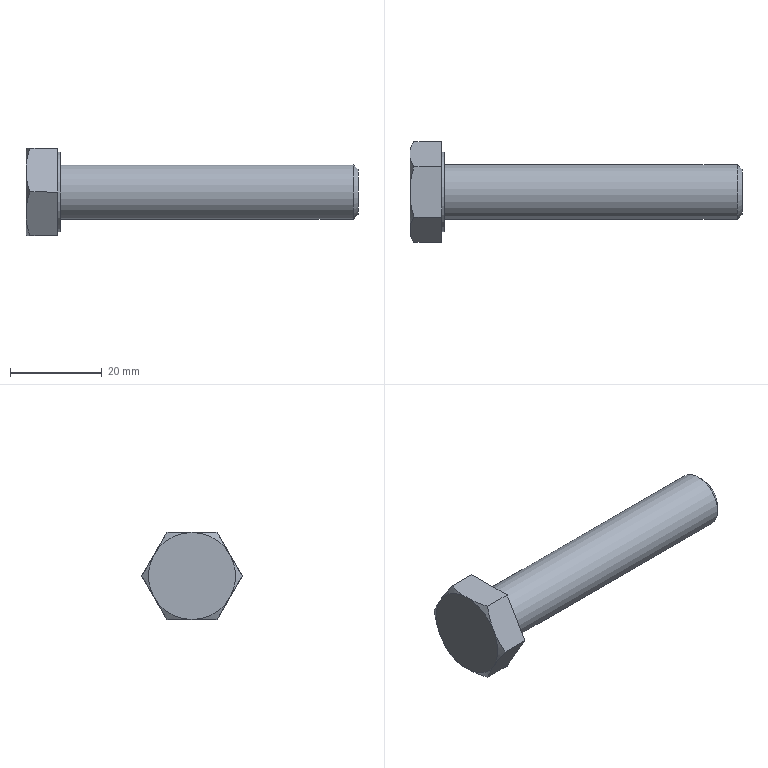Part | STEP file | DIN 931-1 - M12 x 65 | 1 solid | 19 faces | box 72.5 x 21.939 x 19 mm | volume 9623 mm3 | plane 10 | cone 7 | cylinder 2 | commonest cylinder face diameters 12 x1 17.4 x1